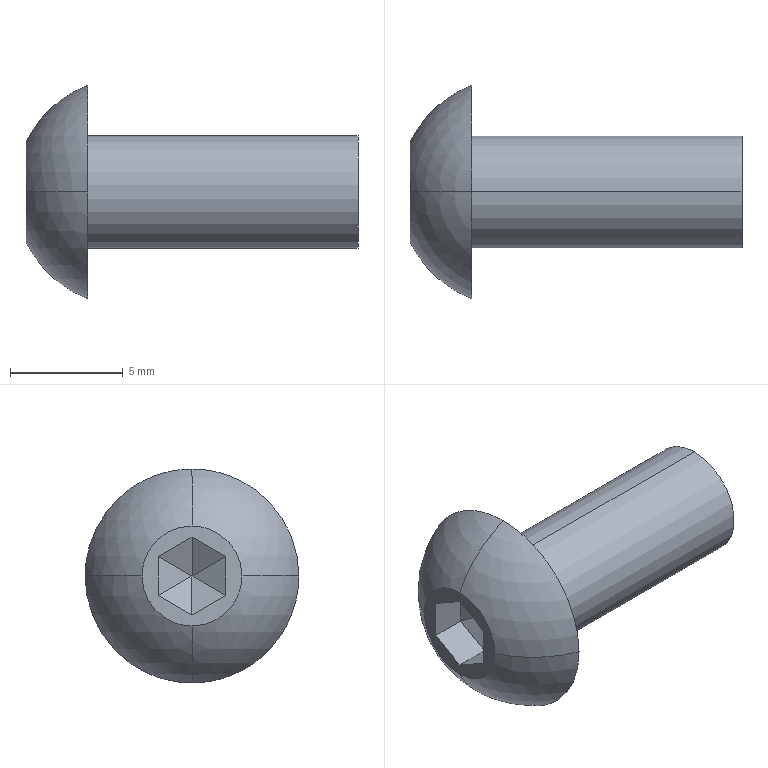Part | STEP file | PN_0005_Default<As Machined> | 1 solid | 21 faces | box 14.75 x 9.5 x 9.5 mm | volume 350.853 mm3 | plane 15 | sphere 4 | cylinder 2 | commonest cylinder face diameters 5 x2
STEP:
#1=CARTESIAN_POINT('',(0.,0.,-2.22));
#2=VERTEX_POINT('',#1);
#3=CARTESIAN_POINT('',(2.75,0.,-4.75));
#4=VERTEX_POINT('',#3);
#5=CARTESIAN_POINT('',(4.581,0.,0.));
#6=DIRECTION('',(0.,-1.,0.));
#7=AXIS2_PLACEMENT_3D('',#5,#6,$);
#8=CIRCLE('',#7,5.091);
#9=EDGE_CURVE('',#2,#4,#8,.T.);
#10=ORIENTED_EDGE('',*,*,#9,.T.);
#11=CARTESIAN_POINT('',(2.75,-4.75,0.));
#12=VERTEX_POINT('',#11);
#13=CARTESIAN_POINT('',(2.75,0.,-4.75));
#14=CARTESIAN_POINT('',(2.75,-0.198,-4.75));
#15=CARTESIAN_POINT('',(2.75,-0.396,-4.74));
#16=CARTESIAN_POINT('',(2.75,-0.6026,-4.719));
#17=CARTESIAN_POINT('',(2.75,-0.9841,-4.66));
#18=CARTESIAN_POINT('',(2.75,-1.435,-4.535));
#19=CARTESIAN_POINT('',(2.75,-1.637,-4.468));
#20=CARTESIAN_POINT('',(2.75,-2.105,-4.279));
#21=CARTESIAN_POINT('',(2.75,-2.607,-3.99));
#22=CARTESIAN_POINT('',(2.75,-2.877,-3.801));
#23=CARTESIAN_POINT('',(2.75,-3.687,-3.12));
#24=CARTESIAN_POINT('',(2.75,-4.315,-2.196));
#25=CARTESIAN_POINT('',(2.75,-4.604,-1.491));
#26=CARTESIAN_POINT('',(2.75,-4.75,-0.7453));
#27=CARTESIAN_POINT('',(2.75,-4.75,0.));
#28=B_SPLINE_CURVE_WITH_KNOTS('',5,(#13,#14,#15,#16,#17,#18,#19,#20,#21,#22,#23,#24,#25,#26,#27),.UNSPECIFIED.,.F.,.U.,(6,3,3,3,6),(0.,2.925,5.015,7.459,12.728),.UNSPECIFIED.);
#29=EDGE_CURVE('',#4,#12,#28,.T.);
#30=ORIENTED_EDGE('',*,*,#29,.T.);
#31=CARTESIAN_POINT('',(0.,-2.22,0.));
#32=VERTEX_POINT('',#31);
#33=CARTESIAN_POINT('',(4.581,0.,0.));
#34=DIRECTION('',(0.,0.,-1.));
#35=AXIS2_PLACEMENT_3D('',#33,#34,$);
#36=CIRCLE('',#35,5.091);
#37=EDGE_CURVE('',#12,#32,#36,.T.);
#38=ORIENTED_EDGE('',*,*,#37,.T.);
#39=CARTESIAN_POINT('',(0.,0.,-2.22));
#40=CARTESIAN_POINT('',(0.,-0.673,-2.22));
#41=CARTESIAN_POINT('',(-0.000003065,-1.345,-1.974));
#42=CARTESIAN_POINT('',(0.00000133,-1.94,-1.428));
#43=CARTESIAN_POINT('',(0.,-2.22,-0.7114));
#44=CARTESIAN_POINT('',(0.,-2.22,0.));
#45=B_SPLINE_CURVE_WITH_KNOTS('',5,(#39,#40,#41,#42,#43,#44),.UNSPECIFIED.,.F.,.U.,(6,6),(0.,5.03),.UNSPECIFIED.);
#46=EDGE_CURVE('',#2,#32,#45,.T.);
#47=ORIENTED_EDGE('',*,*,#46,.F.);
#48=EDGE_LOOP('',(#10,#30,#38,#47));
#49=FACE_OUTER_BOUND('',#48,.T.);
#50=CARTESIAN_POINT('',(4.581,0.,0.));
#51=DIRECTION('',(0.,0.,-1.));
#52=DIRECTION('',(0.,-1.,0.));
#53=AXIS2_PLACEMENT_3D('',#50,#51,#52);
#54=SPHERICAL_SURFACE('',#53,5.091);
#55=ADVANCED_FACE('',(#49),#54,.T.);
#56=ORIENTED_EDGE('',*,*,#9,.F.);
#57=CARTESIAN_POINT('',(0.,2.22,0.));
#58=VERTEX_POINT('',#57);
#59=CARTESIAN_POINT('',(0.,2.22,0.));
#60=CARTESIAN_POINT('',(0.,2.22,-0.7114));
#61=CARTESIAN_POINT('',(0.000000008,1.94,-1.428));
#62=CARTESIAN_POINT('',(-0.000001286,1.345,-1.974));
#63=CARTESIAN_POINT('',(0.,0.673,-2.22));
#64=CARTESIAN_POINT('',(0.,0.,-2.22));
#65=B_SPLINE_CURVE_WITH_KNOTS('',5,(#59,#60,#61,#62,#63,#64),.UNSPECIFIED.,.F.,.U.,(6,6),(0.,5.031),.UNSPECIFIED.);
#66=EDGE_CURVE('',#58,#2,#65,.T.);
#67=ORIENTED_EDGE('',*,*,#66,.F.);
#68=CARTESIAN_POINT('',(2.75,4.75,0.));
#69=VERTEX_POINT('',#68);
#70=CARTESIAN_POINT('',(4.581,0.,0.));
#71=DIRECTION('',(0.,0.,-1.));
#72=AXIS2_PLACEMENT_3D('',#70,#71,$);
#73=CIRCLE('',#72,5.091);
#74=EDGE_CURVE('',#69,#58,#73,.F.);
#75=ORIENTED_EDGE('',*,*,#74,.F.);
#76=CARTESIAN_POINT('',(2.75,4.75,0.));
#77=CARTESIAN_POINT('',(2.75,4.75,-0.7504));
#78=CARTESIAN_POINT('',(2.75,4.602,-1.501));
#79=CARTESIAN_POINT('',(2.75,4.309,-2.211));
#80=CARTESIAN_POINT('',(2.75,3.673,-3.138));
#81=CARTESIAN_POINT('',(2.75,2.856,-3.817));
#82=CARTESIAN_POINT('',(2.75,2.584,-4.004));
#83=CARTESIAN_POINT('',(2.75,2.081,-4.291));
#84=CARTESIAN_POINT('',(2.75,1.612,-4.477));
#85=CARTESIAN_POINT('',(2.75,1.41,-4.542));
#86=CARTESIAN_POINT('',(2.75,0.9666,-4.663));
#87=CARTESIAN_POINT('',(2.75,0.5901,-4.72));
#88=CARTESIAN_POINT('',(2.75,0.3881,-4.74));
#89=CARTESIAN_POINT('',(2.75,0.194,-4.75));
#90=CARTESIAN_POINT('',(2.75,0.,-4.75));
#91=B_SPLINE_CURVE_WITH_KNOTS('',5,(#76,#77,#78,#79,#80,#81,#82,#83,#84,#85,#86,#87,#88,#89,#90),.UNSPECIFIED.,.F.,.U.,(6,3,3,3,6),(0.,5.306,7.756,9.862,12.728),.UNSPECIFIED.);
#92=EDGE_CURVE('',#69,#4,#91,.T.);
#93=ORIENTED_EDGE('',*,*,#92,.T.);
#94=EDGE_LOOP('',(#56,#67,#75,#93));
#95=FACE_OUTER_BOUND('',#94,.T.);
#96=CARTESIAN_POINT('',(4.581,0.,0.));
#97=DIRECTION('',(0.,0.,-1.));
#98=DIRECTION('',(-1.,0.,0.));
#99=AXIS2_PLACEMENT_3D('',#96,#97,#98);
#100=SPHERICAL_SURFACE('',#99,5.091);
#101=ADVANCED_FACE('',(#95),#100,.T.);
#102=ORIENTED_EDGE('',*,*,#29,.F.);
#103=ORIENTED_EDGE('',*,*,#92,.F.);
#104=CARTESIAN_POINT('',(2.75,0.,4.75));
#105=VERTEX_POINT('',#104);
#106=CARTESIAN_POINT('',(2.75,0.,4.75));
#107=CARTESIAN_POINT('',(2.75,0.1093,4.75));
#108=CARTESIAN_POINT('',(2.75,0.2186,4.747));
#109=CARTESIAN_POINT('',(2.75,0.3278,4.741));
#110=CARTESIAN_POINT('',(2.75,0.9688,4.685));
#111=CARTESIAN_POINT('',(2.75,1.597,4.522));
#112=CARTESIAN_POINT('',(2.75,2.097,4.313));
#113=CARTESIAN_POINT('',(2.75,3.023,3.761));
#114=CARTESIAN_POINT('',(2.75,3.761,2.975));
#115=CARTESIAN_POINT('',(2.75,4.072,2.532));
#116=CARTESIAN_POINT('',(2.75,4.462,1.769));
#117=CARTESIAN_POINT('',(2.75,4.672,0.9428));
#118=CARTESIAN_POINT('',(2.75,4.724,0.6305));
#119=CARTESIAN_POINT('',(2.75,4.75,0.3152));
#120=CARTESIAN_POINT('',(2.75,4.75,0.));
#121=B_SPLINE_CURVE_WITH_KNOTS('',5,(#106,#107,#108,#109,#110,#111,#112,#113,#114,#115,#116,#117,#118,#119,#120),.UNSPECIFIED.,.F.,.U.,(6,3,3,3,6),(10.552,11.325,15.099,18.874,21.103),.UNSPECIFIED.);
#122=EDGE_CURVE('',#105,#69,#121,.T.);
#123=ORIENTED_EDGE('',*,*,#122,.F.);
#124=CARTESIAN_POINT('',(2.75,-4.75,0.));
#125=CARTESIAN_POINT('',(2.75,-4.75,0.5338));
#126=CARTESIAN_POINT('',(2.75,-4.675,1.068));
#127=CARTESIAN_POINT('',(2.75,-4.525,1.588));
#128=CARTESIAN_POINT('',(2.75,-4.083,2.571));
#129=CARTESIAN_POINT('',(2.75,-3.387,3.395));
#130=CARTESIAN_POINT('',(2.75,-2.983,3.754));
#131=CARTESIAN_POINT('',(2.75,-2.177,4.29));
#132=CARTESIAN_POINT('',(2.75,-1.267,4.608));
#133=CARTESIAN_POINT('',(2.75,-0.8491,4.703));
#134=CARTESIAN_POINT('',(2.75,-0.4245,4.75));
#135=CARTESIAN_POINT('',(2.75,0.,4.75));
#136=B_SPLINE_CURVE_WITH_KNOTS('',5,(#124,#125,#126,#127,#128,#129,#130,#131,#132,#133,#134,#135),.UNSPECIFIED.,.F.,.U.,(6,3,3,6),(0.,3.775,7.55,10.552),.UNSPECIFIED.);
#137=EDGE_CURVE('',#12,#105,#136,.T.);
#138=ORIENTED_EDGE('',*,*,#137,.F.);
#139=EDGE_LOOP('',(#102,#103,#123,#138));
#140=FACE_OUTER_BOUND('',#139,.T.);
#141=CARTESIAN_POINT('',(2.75,0.,2.5));
#142=VERTEX_POINT('',#141);
#143=CARTESIAN_POINT('',(2.75,0.,-2.5));
#144=VERTEX_POINT('',#143);
#145=CARTESIAN_POINT('',(2.75,0.,0.));
#146=DIRECTION('',(1.,0.,0.));
#147=AXIS2_PLACEMENT_3D('',#145,#146,$);
#148=CIRCLE('',#147,2.5);
#149=EDGE_CURVE('',#142,#144,#148,.T.);
#150=ORIENTED_EDGE('',*,*,#149,.F.);
#151=CARTESIAN_POINT('',(2.75,0.,0.));
#152=DIRECTION('',(1.,0.,0.));
#153=AXIS2_PLACEMENT_3D('',#151,#152,$);
#154=CIRCLE('',#153,2.5);
#155=EDGE_CURVE('',#144,#142,#154,.T.);
#156=ORIENTED_EDGE('',*,*,#155,.F.);
#157=EDGE_LOOP('',(#150,#156));
#158=FACE_BOUND('',#157,.T.);
#159=CARTESIAN_POINT('',(2.75,0.,0.));
#160=DIRECTION('',(1.,0.,0.));
#161=DIRECTION('',(0.,0.,-1.));
#162=AXIS2_PLACEMENT_3D('',#159,#160,#161);
#163=PLANE('',#162);
#164=ADVANCED_FACE('',(#140,#158),#163,.T.);
#165=CARTESIAN_POINT('',(0.,0.,2.22));
#166=VERTEX_POINT('',#165);
#167=CARTESIAN_POINT('',(4.581,0.,0.));
#168=DIRECTION('',(0.,-1.,0.));
#169=AXIS2_PLACEMENT_3D('',#167,#168,$);
#170=CIRCLE('',#169,5.091);
#171=EDGE_CURVE('',#105,#166,#170,.T.);
#172=ORIENTED_EDGE('',*,*,#171,.T.);
#173=CARTESIAN_POINT('',(0.,-2.22,0.));
#174=CARTESIAN_POINT('',(0.,-2.22,0.7114));
#175=CARTESIAN_POINT('',(0.000000008,-1.94,1.428));
#176=CARTESIAN_POINT('',(-0.000001286,-1.345,1.974));
#177=CARTESIAN_POINT('',(0.,-0.673,2.22));
#178=CARTESIAN_POINT('',(0.,0.,2.22));
#179=B_SPLINE_CURVE_WITH_KNOTS('',5,(#173,#174,#175,#176,#177,#178),.UNSPECIFIED.,.F.,.U.,(6,6),(0.,5.031),.UNSPECIFIED.);
#180=EDGE_CURVE('',#32,#166,#179,.T.);
#181=ORIENTED_EDGE('',*,*,#180,.F.);
#182=ORIENTED_EDGE('',*,*,#37,.F.);
#183=ORIENTED_EDGE('',*,*,#137,.T.);
#184=EDGE_LOOP('',(#172,#181,#182,#183));
#185=FACE_OUTER_BOUND('',#184,.T.);
#186=CARTESIAN_POINT('',(4.581,0.,0.));
#187=DIRECTION('',(0.,0.,-1.));
#188=DIRECTION('',(0.,-1.,0.));
#189=AXIS2_PLACEMENT_3D('',#186,#187,#188);
#190=SPHERICAL_SURFACE('',#189,5.091);
#191=ADVANCED_FACE('',(#185),#190,.T.);
#192=ORIENTED_EDGE('',*,*,#66,.T.);
#193=ORIENTED_EDGE('',*,*,#46,.T.);
#194=ORIENTED_EDGE('',*,*,#180,.T.);
#195=CARTESIAN_POINT('',(0.,0.,2.22));
#196=CARTESIAN_POINT('',(0.,0.1785,2.22));
#197=CARTESIAN_POINT('',(0.,0.357,2.202));
#198=CARTESIAN_POINT('',(0.,0.5331,2.166));
#199=CARTESIAN_POINT('',(0.,0.9145,2.047));
#200=CARTESIAN_POINT('',(0.,1.261,1.847));
#201=CARTESIAN_POINT('',(0.,1.437,1.713));
#202=CARTESIAN_POINT('',(0.,1.753,1.405));
#203=CARTESIAN_POINT('',(0.,1.985,1.03));
#204=CARTESIAN_POINT('',(0.,2.077,0.8285));
#205=CARTESIAN_POINT('',(0.,2.168,0.5403));
#206=CARTESIAN_POINT('',(0.,2.209,0.2429));
#207=CARTESIAN_POINT('',(0.,2.216,0.1619));
#208=CARTESIAN_POINT('',(0.,2.22,0.08093));
#209=CARTESIAN_POINT('',(0.,2.22,0.));
#210=B_SPLINE_CURVE_WITH_KNOTS('',5,(#195,#196,#197,#198,#199,#200,#201,#202,#203,#204,#205,#206,#207,#208,#209),.UNSPECIFIED.,.F.,.U.,(6,3,3,3,6),(4.932,6.194,7.742,9.29,9.863),.UNSPECIFIED.);
#211=EDGE_CURVE('',#166,#58,#210,.T.);
#212=ORIENTED_EDGE('',*,*,#211,.T.);
#213=EDGE_LOOP('',(#192,#193,#194,#212));
#214=FACE_OUTER_BOUND('',#213,.T.);
#215=CARTESIAN_POINT('',(0.,-1.5,-0.866));
#216=VERTEX_POINT('',#215);
#217=CARTESIAN_POINT('',(0.,0.,-1.732));
#218=VERTEX_POINT('',#217);
#219=CARTESIAN_POINT('',(0.,-0.75,-1.299));
#220=DIRECTION('',(0.,0.866,-0.5));
#221=VECTOR('',#220,1.);
#222=LINE('',#219,#221);
#223=EDGE_CURVE('',#216,#218,#222,.T.);
#224=ORIENTED_EDGE('',*,*,#223,.T.);
#225=CARTESIAN_POINT('',(0.,1.5,-0.866));
#226=VERTEX_POINT('',#225);
#227=CARTESIAN_POINT('',(0.,0.75,-1.299));
#228=DIRECTION('',(0.,0.866,0.5));
#229=VECTOR('',#228,1.);
#230=LINE('',#227,#229);
#231=EDGE_CURVE('',#218,#226,#230,.T.);
#232=ORIENTED_EDGE('',*,*,#231,.T.);
#233=CARTESIAN_POINT('',(0.,1.5,0.866));
#234=VERTEX_POINT('',#233);
#235=CARTESIAN_POINT('',(0.,1.5,0.));
#236=DIRECTION('',(0.,0.,1.));
#237=VECTOR('',#236,1.);
#238=LINE('',#235,#237);
#239=EDGE_CURVE('',#226,#234,#238,.T.);
#240=ORIENTED_EDGE('',*,*,#239,.T.);
#241=CARTESIAN_POINT('',(0.,0.,1.732));
#242=VERTEX_POINT('',#241);
#243=CARTESIAN_POINT('',(0.,0.75,1.299));
#244=DIRECTION('',(0.,-0.866,0.5));
#245=VECTOR('',#244,1.);
#246=LINE('',#243,#245);
#247=EDGE_CURVE('',#234,#242,#246,.T.);
#248=ORIENTED_EDGE('',*,*,#247,.T.);
#249=CARTESIAN_POINT('',(0.,-1.5,0.866));
#250=VERTEX_POINT('',#249);
#251=CARTESIAN_POINT('',(0.,-0.75,1.299));
#252=DIRECTION('',(0.,-0.866,-0.5));
#253=VECTOR('',#252,1.);
#254=LINE('',#251,#253);
#255=EDGE_CURVE('',#242,#250,#254,.T.);
#256=ORIENTED_EDGE('',*,*,#255,.T.);
#257=CARTESIAN_POINT('',(0.,-1.5,0.));
#258=DIRECTION('',(0.,0.,-1.));
#259=VECTOR('',#258,1.);
#260=LINE('',#257,#259);
#261=EDGE_CURVE('',#250,#216,#260,.T.);
#262=ORIENTED_EDGE('',*,*,#261,.T.);
#263=EDGE_LOOP('',(#224,#232,#240,#248,#256,#262));
#264=FACE_BOUND('',#263,.T.);
#265=CARTESIAN_POINT('',(0.,0.,0.));
#266=DIRECTION('',(1.,0.,0.));
#267=DIRECTION('',(0.,0.,-1.));
#268=AXIS2_PLACEMENT_3D('',#265,#266,#267);
#269=PLANE('',#268);
#270=ADVANCED_FACE('',(#214,#264),#269,.F.);
#271=ORIENTED_EDGE('',*,*,#171,.F.);
#272=ORIENTED_EDGE('',*,*,#122,.T.);
#273=ORIENTED_EDGE('',*,*,#74,.T.);
#274=ORIENTED_EDGE('',*,*,#211,.F.);
#275=EDGE_LOOP('',(#271,#272,#273,#274));
#276=FACE_OUTER_BOUND('',#275,.T.);
#277=CARTESIAN_POINT('',(4.581,0.,0.));
#278=DIRECTION('',(0.,0.,-1.));
#279=DIRECTION('',(-1.,0.,0.));
#280=AXIS2_PLACEMENT_3D('',#277,#278,#279);
#281=SPHERICAL_SURFACE('',#280,5.091);
#282=ADVANCED_FACE('',(#276),#281,.T.);
#283=CARTESIAN_POINT('',(14.75,0.,-2.5));
#284=VERTEX_POINT('',#283);
#285=CARTESIAN_POINT('',(14.75,0.,-2.5));
#286=DIRECTION('',(-1.,0.,0.));
#287=VECTOR('',#286,1.);
#288=LINE('',#285,#287);
#289=EDGE_CURVE('',#284,#144,#288,.T.);
#290=ORIENTED_EDGE('',*,*,#289,.F.);
#291=CARTESIAN_POINT('',(14.75,0.,2.5));
#292=VERTEX_POINT('',#291);
#293=CARTESIAN_POINT('',(14.75,0.,0.));
#294=DIRECTION('',(-1.,0.,0.));
#295=AXIS2_PLACEMENT_3D('',#293,#294,$);
#296=CIRCLE('',#295,2.5);
#297=EDGE_CURVE('',#292,#284,#296,.F.);
#298=ORIENTED_EDGE('',*,*,#297,.F.);
#299=CARTESIAN_POINT('',(14.75,0.,2.5));
#300=DIRECTION('',(-1.,0.,0.));
#301=VECTOR('',#300,1.);
#302=LINE('',#299,#301);
#303=EDGE_CURVE('',#292,#142,#302,.T.);
#304=ORIENTED_EDGE('',*,*,#303,.T.);
#305=ORIENTED_EDGE('',*,*,#149,.T.);
#306=EDGE_LOOP('',(#290,#298,#304,#305));
#307=FACE_OUTER_BOUND('',#306,.T.);
#308=CARTESIAN_POINT('',(14.75,0.,0.));
#309=DIRECTION('',(-1.,0.,0.));
#310=DIRECTION('',(0.,0.,-1.));
#311=AXIS2_PLACEMENT_3D('',#308,#309,#310);
#312=CYLINDRICAL_SURFACE('',#311,2.5);
#313=ADVANCED_FACE('',(#307),#312,.T.);
#314=CARTESIAN_POINT('',(14.75,0.,0.));
#315=DIRECTION('',(-1.,0.,0.));
#316=AXIS2_PLACEMENT_3D('',#314,#315,$);
#317=CIRCLE('',#316,2.5);
#318=EDGE_CURVE('',#284,#292,#317,.F.);
#319=ORIENTED_EDGE('',*,*,#318,.F.);
#320=ORIENTED_EDGE('',*,*,#289,.T.);
#321=ORIENTED_EDGE('',*,*,#155,.T.);
#322=ORIENTED_EDGE('',*,*,#303,.F.);
#323=EDGE_LOOP('',(#319,#320,#321,#322));
#324=FACE_OUTER_BOUND('',#323,.T.);
#325=CARTESIAN_POINT('',(14.75,0.,0.));
#326=DIRECTION('',(-1.,0.,0.));
#327=DIRECTION('',(0.,0.,1.));
#328=AXIS2_PLACEMENT_3D('',#325,#326,#327);
#329=CYLINDRICAL_SURFACE('',#328,2.5);
#330=ADVANCED_FACE('',(#324),#329,.T.);
#331=ORIENTED_EDGE('',*,*,#223,.F.);
#332=CARTESIAN_POINT('',(1.56,-1.5,-0.866));
#333=VERTEX_POINT('',#332);
#334=CARTESIAN_POINT('',(0.78,-1.5,-0.866));
#335=DIRECTION('',(-1.,0.,0.));
#336=VECTOR('',#335,1.);
#337=LINE('',#334,#336);
#338=EDGE_CURVE('',#333,#216,#337,.T.);
#339=ORIENTED_EDGE('',*,*,#338,.F.);
#340=CARTESIAN_POINT('',(1.56,0.000000001,-1.732));
#341=VERTEX_POINT('',#340);
#342=CARTESIAN_POINT('',(1.56,-0.75,-1.299));
#343=DIRECTION('',(0.,0.866,-0.5));
#344=VECTOR('',#343,1.);
#345=LINE('',#342,#344);
#346=EDGE_CURVE('',#333,#341,#345,.T.);
#347=ORIENTED_EDGE('',*,*,#346,.T.);
#348=CARTESIAN_POINT('',(0.78,0.000000001,-1.732));
#349=DIRECTION('',(-1.,0.,0.));
#350=VECTOR('',#349,1.);
#351=LINE('',#348,#350);
#352=EDGE_CURVE('',#341,#218,#351,.T.);
#353=ORIENTED_EDGE('',*,*,#352,.T.);
#354=EDGE_LOOP('',(#331,#339,#347,#353));
#355=FACE_OUTER_BOUND('',#354,.T.);
#356=CARTESIAN_POINT('',(1.56,-1.5,-0.866));
#357=DIRECTION('',(0.,0.5,0.866));
#358=DIRECTION('',(0.,-0.866,0.5));
#359=AXIS2_PLACEMENT_3D('',#356,#357,#358);
#360=PLANE('',#359);
#361=ADVANCED_FACE('',(#355),#360,.T.);
#362=ORIENTED_EDGE('',*,*,#231,.F.);
#363=ORIENTED_EDGE('',*,*,#352,.F.);
#364=CARTESIAN_POINT('',(1.56,1.5,-0.866));
#365=VERTEX_POINT('',#364);
#366=CARTESIAN_POINT('',(1.56,0.75,-1.299));
#367=DIRECTION('',(0.,0.866,0.5));
#368=VECTOR('',#367,1.);
#369=LINE('',#366,#368);
#370=EDGE_CURVE('',#341,#365,#369,.T.);
#371=ORIENTED_EDGE('',*,*,#370,.T.);
#372=CARTESIAN_POINT('',(0.78,1.5,-0.866));
#373=DIRECTION('',(-1.,0.,0.));
#374=VECTOR('',#373,1.);
#375=LINE('',#372,#374);
#376=EDGE_CURVE('',#365,#226,#375,.T.);
#377=ORIENTED_EDGE('',*,*,#376,.T.);
#378=EDGE_LOOP('',(#362,#363,#371,#377));
#379=FACE_OUTER_BOUND('',#378,.T.);
#380=CARTESIAN_POINT('',(1.56,0.,-1.732));
#381=DIRECTION('',(0.,-0.5,0.866));
#382=DIRECTION('',(0.,-0.866,-0.5));
#383=AXIS2_PLACEMENT_3D('',#380,#381,#382);
#384=PLANE('',#383);
#385=ADVANCED_FACE('',(#379),#384,.T.);
#386=ORIENTED_EDGE('',*,*,#239,.F.);
#387=ORIENTED_EDGE('',*,*,#376,.F.);
#388=CARTESIAN_POINT('',(1.56,1.5,0.866));
#389=VERTEX_POINT('',#388);
#390=CARTESIAN_POINT('',(1.56,1.5,0.));
#391=DIRECTION('',(0.,0.,1.));
#392=VECTOR('',#391,1.);
#393=LINE('',#390,#392);
#394=EDGE_CURVE('',#365,#389,#393,.T.);
#395=ORIENTED_EDGE('',*,*,#394,.T.);
#396=CARTESIAN_POINT('',(0.78,1.5,0.866));
#397=DIRECTION('',(-1.,0.,0.));
#398=VECTOR('',#397,1.);
#399=LINE('',#396,#398);
#400=EDGE_CURVE('',#389,#234,#399,.T.);
#401=ORIENTED_EDGE('',*,*,#400,.T.);
#402=EDGE_LOOP('',(#386,#387,#395,#401));
#403=FACE_OUTER_BOUND('',#402,.T.);
#404=CARTESIAN_POINT('',(1.56,1.5,-0.866));
#405=DIRECTION('',(0.,-1.,0.));
#406=DIRECTION('',(0.,0.,-1.));
#407=AXIS2_PLACEMENT_3D('',#404,#405,#406);
#408=PLANE('',#407);
#409=ADVANCED_FACE('',(#403),#408,.T.);
#410=ORIENTED_EDGE('',*,*,#247,.F.);
#411=ORIENTED_EDGE('',*,*,#400,.F.);
#412=CARTESIAN_POINT('',(1.56,-0.000000001,1.732));
#413=VERTEX_POINT('',#412);
#414=CARTESIAN_POINT('',(1.56,0.75,1.299));
#415=DIRECTION('',(0.,-0.866,0.5));
#416=VECTOR('',#415,1.);
#417=LINE('',#414,#416);
#418=EDGE_CURVE('',#389,#413,#417,.T.);
#419=ORIENTED_EDGE('',*,*,#418,.T.);
#420=CARTESIAN_POINT('',(0.78,-0.000000001,1.732));
#421=DIRECTION('',(-1.,0.,0.));
#422=VECTOR('',#421,1.);
#423=LINE('',#420,#422);
#424=EDGE_CURVE('',#413,#242,#423,.T.);
#425=ORIENTED_EDGE('',*,*,#424,.T.);
#426=EDGE_LOOP('',(#410,#411,#419,#425));
#427=FACE_OUTER_BOUND('',#426,.T.);
#428=CARTESIAN_POINT('',(1.56,1.5,0.866));
#429=DIRECTION('',(0.,-0.5,-0.866));
#430=DIRECTION('',(0.,0.866,-0.5));
#431=AXIS2_PLACEMENT_3D('',#428,#429,#430);
#432=PLANE('',#431);
#433=ADVANCED_FACE('',(#427),#432,.T.);
#434=ORIENTED_EDGE('',*,*,#255,.F.);
#435=ORIENTED_EDGE('',*,*,#424,.F.);
#436=CARTESIAN_POINT('',(1.56,-1.5,0.866));
#437=VERTEX_POINT('',#436);
#438=CARTESIAN_POINT('',(1.56,-0.75,1.299));
#439=DIRECTION('',(0.,-0.866,-0.5));
#440=VECTOR('',#439,1.);
#441=LINE('',#438,#440);
#442=EDGE_CURVE('',#413,#437,#441,.T.);
#443=ORIENTED_EDGE('',*,*,#442,.T.);
#444=CARTESIAN_POINT('',(0.78,-1.5,0.866));
#445=DIRECTION('',(-1.,0.,0.));
#446=VECTOR('',#445,1.);
#447=LINE('',#444,#446);
#448=EDGE_CURVE('',#437,#250,#447,.T.);
#449=ORIENTED_EDGE('',*,*,#448,.T.);
#450=EDGE_LOOP('',(#434,#435,#443,#449));
#451=FACE_OUTER_BOUND('',#450,.T.);
#452=CARTESIAN_POINT('',(1.56,0.,1.732));
#453=DIRECTION('',(0.,0.5,-0.866));
#454=DIRECTION('',(0.,0.866,0.5));
#455=AXIS2_PLACEMENT_3D('',#452,#453,#454);
#456=PLANE('',#455);
#457=ADVANCED_FACE('',(#451),#456,.T.);
#458=ORIENTED_EDGE('',*,*,#261,.F.);
#459=ORIENTED_EDGE('',*,*,#448,.F.);
#460=CARTESIAN_POINT('',(1.56,-1.5,0.));
#461=DIRECTION('',(0.,0.,-1.));
#462=VECTOR('',#461,1.);
#463=LINE('',#460,#462);
#464=EDGE_CURVE('',#437,#333,#463,.T.);
#465=ORIENTED_EDGE('',*,*,#464,.T.);
#466=ORIENTED_EDGE('',*,*,#338,.T.);
#467=EDGE_LOOP('',(#458,#459,#465,#466));
#468=FACE_OUTER_BOUND('',#467,.T.);
#469=CARTESIAN_POINT('',(1.56,-1.5,0.866));
#470=DIRECTION('',(0.,1.,0.));
#471=DIRECTION('',(0.,0.,1.));
#472=AXIS2_PLACEMENT_3D('',#469,#470,#471);
#473=PLANE('',#472);
#474=ADVANCED_FACE('',(#468),#473,.T.);
#475=ORIENTED_EDGE('',*,*,#297,.T.);
#476=ORIENTED_EDGE('',*,*,#318,.T.);
#477=EDGE_LOOP('',(#475,#476));
#478=FACE_OUTER_BOUND('',#477,.T.);
#479=CARTESIAN_POINT('',(14.75,0.,0.));
#480=DIRECTION('',(1.,0.,0.));
#481=DIRECTION('',(0.,0.,-1.));
#482=AXIS2_PLACEMENT_3D('',#479,#480,#481);
#483=PLANE('',#482);
#484=ADVANCED_FACE('',(#478),#483,.T.);
#485=ORIENTED_EDGE('',*,*,#346,.F.);
#486=CARTESIAN_POINT('',(2.426,0.,-0.000000001));
#487=VERTEX_POINT('',#486);
#488=CARTESIAN_POINT('',(1.993,-0.75,-0.433));
#489=DIRECTION('',(-0.4472,-0.7746,-0.4472));
#490=VECTOR('',#489,1.);
#491=LINE('',#488,#490);
#492=EDGE_CURVE('',#487,#333,#491,.T.);
#493=ORIENTED_EDGE('',*,*,#492,.F.);
#494=CARTESIAN_POINT('',(1.993,-0.000000001,-0.866));
#495=DIRECTION('',(-0.4472,0.,-0.8944));
#496=VECTOR('',#495,1.);
#497=LINE('',#494,#496);
#498=EDGE_CURVE('',#487,#341,#497,.T.);
#499=ORIENTED_EDGE('',*,*,#498,.T.);
#500=EDGE_LOOP('',(#485,#493,#499));
#501=FACE_OUTER_BOUND('',#500,.T.);
#502=CARTESIAN_POINT('',(1.56,-1.5,-0.866));
#503=DIRECTION('',(0.866,-0.25,-0.433));
#504=DIRECTION('',(-0.4472,0.,-0.8944));
#505=AXIS2_PLACEMENT_3D('',#502,#503,#504);
#506=PLANE('',#505);
#507=ADVANCED_FACE('',(#501),#506,.F.);
#508=ORIENTED_EDGE('',*,*,#370,.F.);
#509=ORIENTED_EDGE('',*,*,#498,.F.);
#510=CARTESIAN_POINT('',(1.993,0.75,-0.433));
#511=DIRECTION('',(-0.4472,0.7746,-0.4472));
#512=VECTOR('',#511,1.);
#513=LINE('',#510,#512);
#514=EDGE_CURVE('',#487,#365,#513,.T.);
#515=ORIENTED_EDGE('',*,*,#514,.T.);
#516=EDGE_LOOP('',(#508,#509,#515));
#517=FACE_OUTER_BOUND('',#516,.T.);
#518=CARTESIAN_POINT('',(1.56,0.,-1.732));
#519=DIRECTION('',(0.866,0.25,-0.433));
#520=DIRECTION('',(-0.4472,0.,-0.8944));
#521=AXIS2_PLACEMENT_3D('',#518,#519,#520);
#522=PLANE('',#521);
#523=ADVANCED_FACE('',(#517),#522,.F.);
#524=ORIENTED_EDGE('',*,*,#394,.F.);
#525=ORIENTED_EDGE('',*,*,#514,.F.);
#526=CARTESIAN_POINT('',(1.993,0.75,0.433));
#527=DIRECTION('',(-0.4472,0.7746,0.4472));
#528=VECTOR('',#527,1.);
#529=LINE('',#526,#528);
#530=EDGE_CURVE('',#487,#389,#529,.T.);
#531=ORIENTED_EDGE('',*,*,#530,.T.);
#532=EDGE_LOOP('',(#524,#525,#531));
#533=FACE_OUTER_BOUND('',#532,.T.);
#534=CARTESIAN_POINT('',(1.56,1.5,-0.866));
#535=DIRECTION('',(0.866,0.5,0.));
#536=DIRECTION('',(-0.5,0.866,0.));
#537=AXIS2_PLACEMENT_3D('',#534,#535,#536);
#538=PLANE('',#537);
#539=ADVANCED_FACE('',(#533),#538,.F.);
#540=ORIENTED_EDGE('',*,*,#418,.F.);
#541=ORIENTED_EDGE('',*,*,#530,.F.);
#542=CARTESIAN_POINT('',(1.993,0.000000001,0.866));
#543=DIRECTION('',(-0.4472,0.,0.8944));
#544=VECTOR('',#543,1.);
#545=LINE('',#542,#544);
#546=EDGE_CURVE('',#487,#413,#545,.T.);
#547=ORIENTED_EDGE('',*,*,#546,.T.);
#548=EDGE_LOOP('',(#540,#541,#547));
#549=FACE_OUTER_BOUND('',#548,.T.);
#550=CARTESIAN_POINT('',(1.56,1.5,0.866));
#551=DIRECTION('',(0.866,0.25,0.433));
#552=DIRECTION('',(0.4472,0.,-0.8944));
#553=AXIS2_PLACEMENT_3D('',#550,#551,#552);
#554=PLANE('',#553);
#555=ADVANCED_FACE('',(#549),#554,.F.);
#556=ORIENTED_EDGE('',*,*,#442,.F.);
#557=ORIENTED_EDGE('',*,*,#546,.F.);
#558=CARTESIAN_POINT('',(1.993,-0.75,0.433));
#559=DIRECTION('',(-0.4472,-0.7746,0.4472));
#560=VECTOR('',#559,1.);
#561=LINE('',#558,#560);
#562=EDGE_CURVE('',#487,#437,#561,.T.);
#563=ORIENTED_EDGE('',*,*,#562,.T.);
#564=EDGE_LOOP('',(#556,#557,#563));
#565=FACE_OUTER_BOUND('',#564,.T.);
#566=CARTESIAN_POINT('',(1.56,0.,1.732));
#567=DIRECTION('',(0.866,-0.25,0.433));
#568=DIRECTION('',(0.4472,0.,-0.8944));
#569=AXIS2_PLACEMENT_3D('',#566,#567,#568);
#570=PLANE('',#569);
#571=ADVANCED_FACE('',(#565),#570,.F.);
#572=ORIENTED_EDGE('',*,*,#464,.F.);
#573=ORIENTED_EDGE('',*,*,#562,.F.);
#574=ORIENTED_EDGE('',*,*,#492,.T.);
#575=EDGE_LOOP('',(#572,#573,#574));
#576=FACE_OUTER_BOUND('',#575,.T.);
#577=CARTESIAN_POINT('',(1.56,-1.5,0.866));
#578=DIRECTION('',(0.866,-0.5,0.));
#579=DIRECTION('',(0.5,0.866,0.));
#580=AXIS2_PLACEMENT_3D('',#577,#578,#579);
#581=PLANE('',#580);
#582=ADVANCED_FACE('',(#576),#581,.F.);
#583=CLOSED_SHELL('',(#55,#101,#164,#191,#270,#282,#313,#330,#361,#385,#409,#433,#457,#474,#484,#507,#523,#539,#555,#571,#582));
#584=MANIFOLD_SOLID_BREP('',#583);
#585=(LENGTH_UNIT()NAMED_UNIT(*)SI_UNIT(.MILLI.,.METRE.));
#586=UNCERTAINTY_MEASURE_WITH_UNIT(LENGTH_MEASURE(0.005),#585,'','');
#587=(NAMED_UNIT(*)PLANE_ANGLE_UNIT()SI_UNIT($,.RADIAN.));
#588=(NAMED_UNIT(*)SI_UNIT($,.STERADIAN.)SOLID_ANGLE_UNIT());
#589=(GEOMETRIC_REPRESENTATION_CONTEXT(3)GLOBAL_UNCERTAINTY_ASSIGNED_CONTEXT((#586))GLOBAL_UNIT_ASSIGNED_CONTEXT((#585,#587,#588))REPRESENTATION_CONTEXT('',''));
#590=ADVANCED_BREP_SHAPE_REPRESENTATION('',(#584),#589);